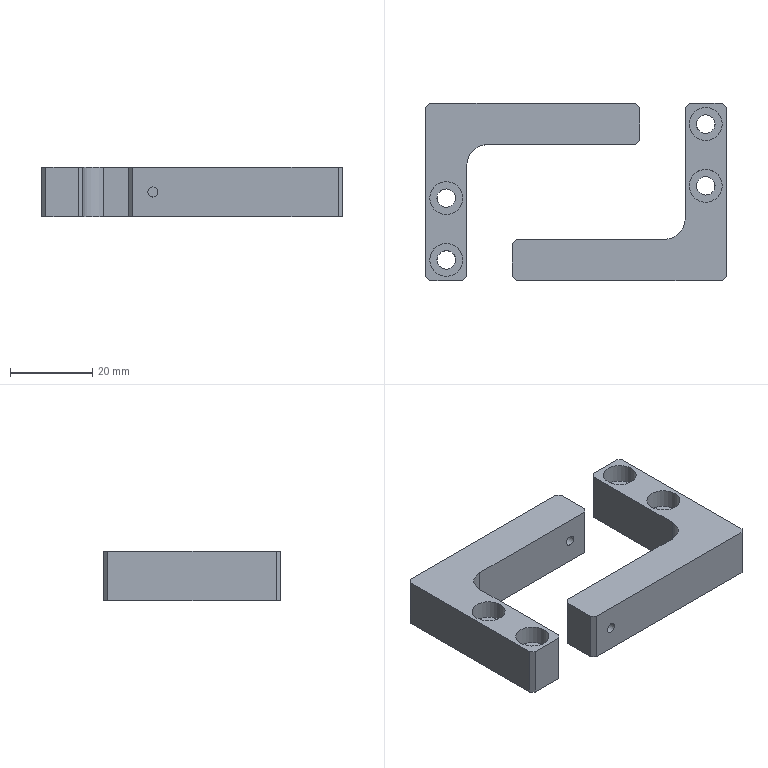CAM job | NX | 3-axis milling, drilling | part box 73 x 43 x 12 mm | stock box 79 x 49 x 12 mm
Tools:
number,name,description,diameter,corner_radius,flute_length,length,flutes
22,D6A45,Milling Tool-5 Parameters,6.0,0.0,3.0,3.0,2
21,4.5ZT,Drilling Tool,3.2,0.0,35.0,50.0,2
20,D10,Milling Tool-5 Parameters,10.0,0.0,50.0,75.0,2
17,D6,Milling Tool-5 Parameters,6.0,0.0,50.0,75.0,2
Operations:
program,operation,operation_type,tool,method,geometry_group,spindle_rpm,surface_speed,feed_per_tooth,feed_cut,feed_plunge,cut_length_mm,path_length_mm,cut_time_min,machine_time_min
1AB胶-80-50-12毛胚,DRILLING_COPY_1_COPY_1,Operation,D6A45,METHOD,A,5000.0,94.0,0.025,250.0,0.0,16.0,194.737,0.064,0.0819
1AB胶-80-50-12毛胚,DRILLING_COPY_1_COPY_COPY_COPY_COPY_1_COPY_COPY_1_COPY_COPY_1,Operation,4.5ZT,METHOD,A,2000.0,20.0,0.0375,150.0,0.0,69.846,304.875,0.4656,0.4891
1AB胶-80-50-12毛胚,ZLEVEL_PROFILE_COPY,ZLevelMilling,D10,METHOD,A,7500.0,235.0,0.1667,2500.0,100.0,6684.423,6857.368,2.674,2.691
1AB胶-80-50-12毛胚,HOLE_MILLING_COPY,CylinderMilling,D6,METHOD,A,7500.0,141.0,0.0933,1400.0,100.0,358.79,814.902,0.2563,0.3019
1AB胶-80-50-12毛胚,ZLEVEL_PROFILE_1_COPY_1_COPY_COPY,ZLevelMilling,D6A45,METHOD,A,7500.0,141.0,0.0667,1000.0,100.0,496.26,1072.551,0.4963,0.5539
1AB胶-80-50-12毛胚,ZLEVEL_PROFILE_COPY_COPY_1,ZLevelMilling,D6,METHOD,A,7500.0,235.0,0.0667,1000.0,100.0,1303.347,1534.013,1.303,1.326